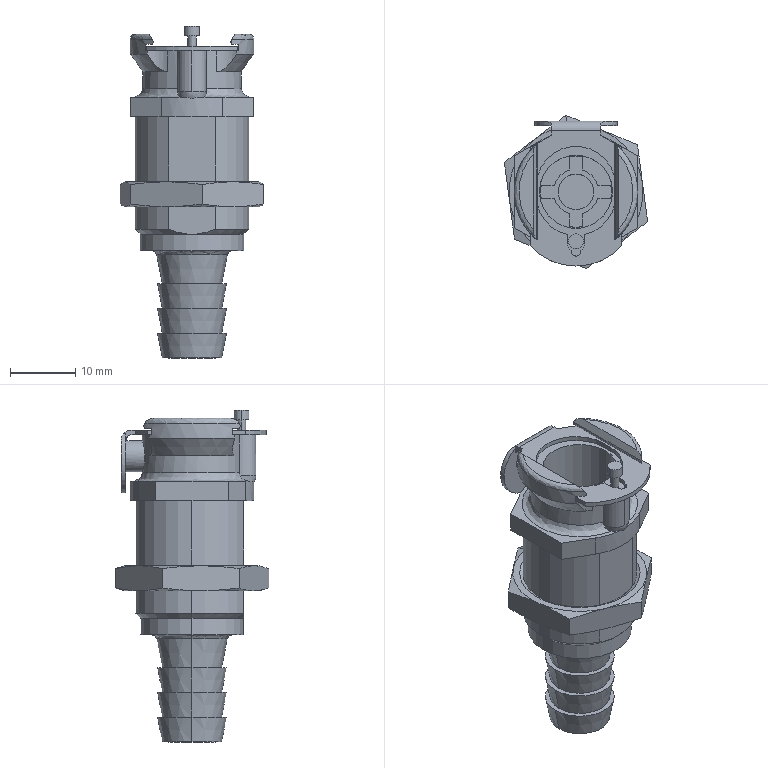Part | SolidWorks | 3 solids | 218 faces | box 22.024 x 23.624 x 51.054 mm | volume 6283 mm3 | plane 115 | cylinder 61 | cone 35 | spline 7 | commonest cylinder face diameters 10.871 x5 6.096 x4 7.01 x4 11.252 x4 19.05 x4 12.192 x3